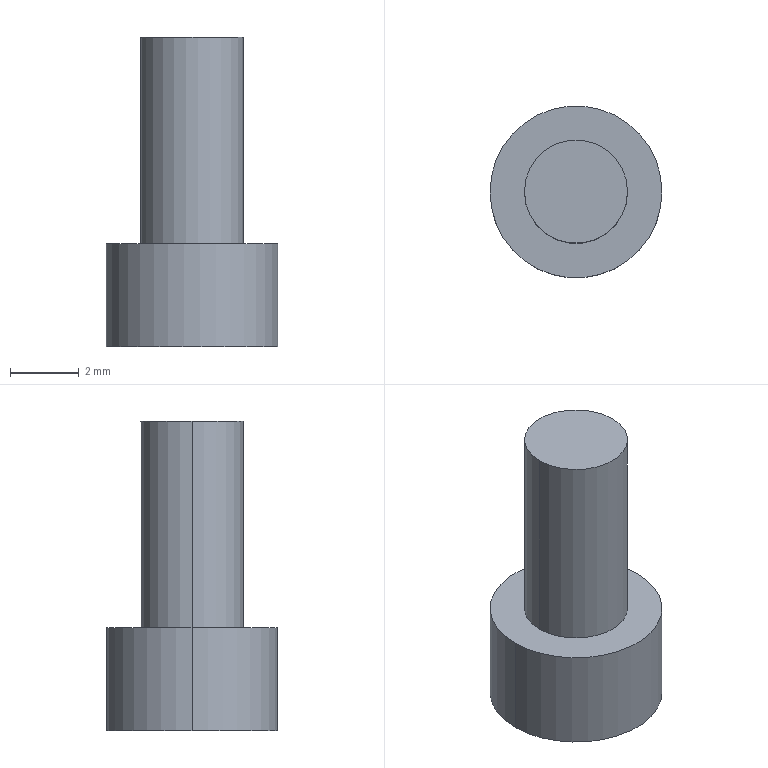Part | SolidWorks | features Extrusion 1, ICE 1 | 1 solid | 7 faces | box 5 x 5 x 9 mm | volume 101.316 mm3 | cylinder 4 | plane 3 | commonest cylinder face diameters 3 x2 5 x2
STEP:
#1=CARTESIAN_POINT('',(1.5,0.,9.));
#2=VERTEX_POINT('',#1);
#3=CARTESIAN_POINT('',(-1.5,0.,9.));
#4=VERTEX_POINT('',#3);
#5=CARTESIAN_POINT('',(0.,0.,9.));
#6=DIRECTION('',(0.,0.,1.));
#7=DIRECTION('',(1.,0.,0.));
#8=AXIS2_PLACEMENT_3D('',#5,#6,#7);
#9=CIRCLE('',#8,1.5);
#10=EDGE_CURVE('',#2,#4,#9,.T.);
#11=ORIENTED_EDGE('',*,*,#10,.F.);
#12=CARTESIAN_POINT('',(1.5,0.,3.));
#13=VERTEX_POINT('',#12);
#14=CARTESIAN_POINT('',(1.5,0.,9.));
#15=DIRECTION('',(0.,0.,-1.));
#16=VECTOR('',#15,1000.);
#17=LINE('',#14,#16);
#18=EDGE_CURVE('',#2,#13,#17,.T.);
#19=ORIENTED_EDGE('',*,*,#18,.T.);
#20=CARTESIAN_POINT('',(-1.5,0.,3.));
#21=VERTEX_POINT('',#20);
#22=CARTESIAN_POINT('',(0.,0.,3.));
#23=DIRECTION('',(0.,0.,1.));
#24=DIRECTION('',(1.,0.,0.));
#25=AXIS2_PLACEMENT_3D('',#22,#23,#24);
#26=CIRCLE('',#25,1.5);
#27=EDGE_CURVE('',#13,#21,#26,.T.);
#28=ORIENTED_EDGE('',*,*,#27,.T.);
#29=CARTESIAN_POINT('',(-1.5,0.,9.));
#30=DIRECTION('',(0.,0.,-1.));
#31=VECTOR('',#30,1000.);
#32=LINE('',#29,#31);
#33=EDGE_CURVE('',#4,#21,#32,.T.);
#34=ORIENTED_EDGE('',*,*,#33,.F.);
#35=EDGE_LOOP('',(#11,#19,#28,#34));
#36=FACE_OUTER_BOUND('',#35,.T.);
#37=CARTESIAN_POINT('',(0.,0.,9.));
#38=DIRECTION('',(0.,0.,-1.));
#39=DIRECTION('',(-1.,0.,0.));
#40=AXIS2_PLACEMENT_3D('',#37,#38,#39);
#41=CYLINDRICAL_SURFACE('',#40,1.5);
#42=ADVANCED_FACE('',(#36),#41,.T.);
#43=CARTESIAN_POINT('',(2.5,0.,3.));
#44=VERTEX_POINT('',#43);
#45=CARTESIAN_POINT('',(-2.5,0.,3.));
#46=VERTEX_POINT('',#45);
#47=CARTESIAN_POINT('',(0.,0.,3.));
#48=DIRECTION('',(0.,0.,1.));
#49=DIRECTION('',(1.,0.,0.));
#50=AXIS2_PLACEMENT_3D('',#47,#48,#49);
#51=CIRCLE('',#50,2.5);
#52=EDGE_CURVE('',#44,#46,#51,.T.);
#53=ORIENTED_EDGE('',*,*,#52,.F.);
#54=CARTESIAN_POINT('',(2.5,0.,0.));
#55=VERTEX_POINT('',#54);
#56=CARTESIAN_POINT('',(2.5,0.,3.));
#57=DIRECTION('',(0.,0.,-1.));
#58=VECTOR('',#57,1000.);
#59=LINE('',#56,#58);
#60=EDGE_CURVE('',#44,#55,#59,.T.);
#61=ORIENTED_EDGE('',*,*,#60,.T.);
#62=CARTESIAN_POINT('',(-2.5,0.,0.));
#63=VERTEX_POINT('',#62);
#64=CARTESIAN_POINT('',(0.,0.,0.));
#65=DIRECTION('',(0.,0.,1.));
#66=DIRECTION('',(1.,0.,0.));
#67=AXIS2_PLACEMENT_3D('',#64,#65,#66);
#68=CIRCLE('',#67,2.5);
#69=EDGE_CURVE('',#55,#63,#68,.T.);
#70=ORIENTED_EDGE('',*,*,#69,.T.);
#71=CARTESIAN_POINT('',(-2.5,0.,3.));
#72=DIRECTION('',(0.,0.,-1.));
#73=VECTOR('',#72,1000.);
#74=LINE('',#71,#73);
#75=EDGE_CURVE('',#46,#63,#74,.T.);
#76=ORIENTED_EDGE('',*,*,#75,.F.);
#77=EDGE_LOOP('',(#53,#61,#70,#76));
#78=FACE_OUTER_BOUND('',#77,.T.);
#79=CARTESIAN_POINT('',(0.,0.,3.));
#80=DIRECTION('',(0.,0.,-1.));
#81=DIRECTION('',(-1.,0.,0.));
#82=AXIS2_PLACEMENT_3D('',#79,#80,#81);
#83=CYLINDRICAL_SURFACE('',#82,2.5);
#84=ADVANCED_FACE('',(#78),#83,.T.);
#85=ORIENTED_EDGE('',*,*,#60,.F.);
#86=CARTESIAN_POINT('',(0.,0.,3.));
#87=DIRECTION('',(0.,0.,1.));
#88=DIRECTION('',(1.,0.,0.));
#89=AXIS2_PLACEMENT_3D('',#86,#87,#88);
#90=CIRCLE('',#89,2.5);
#91=EDGE_CURVE('',#46,#44,#90,.T.);
#92=ORIENTED_EDGE('',*,*,#91,.F.);
#93=ORIENTED_EDGE('',*,*,#75,.T.);
#94=CARTESIAN_POINT('',(0.,0.,0.));
#95=DIRECTION('',(0.,0.,1.));
#96=DIRECTION('',(1.,0.,0.));
#97=AXIS2_PLACEMENT_3D('',#94,#95,#96);
#98=CIRCLE('',#97,2.5);
#99=EDGE_CURVE('',#63,#55,#98,.T.);
#100=ORIENTED_EDGE('',*,*,#99,.T.);
#101=EDGE_LOOP('',(#85,#92,#93,#100));
#102=FACE_OUTER_BOUND('',#101,.T.);
#103=CARTESIAN_POINT('',(0.,0.,3.));
#104=DIRECTION('',(0.,0.,-1.));
#105=DIRECTION('',(-1.,0.,0.));
#106=AXIS2_PLACEMENT_3D('',#103,#104,#105);
#107=CYLINDRICAL_SURFACE('',#106,2.5);
#108=ADVANCED_FACE('',(#102),#107,.T.);
#109=CARTESIAN_POINT('',(0.,0.,3.));
#110=DIRECTION('',(0.,0.,1.));
#111=DIRECTION('',(1.,0.,0.));
#112=AXIS2_PLACEMENT_3D('',#109,#110,#111);
#113=CIRCLE('',#112,1.5);
#114=EDGE_CURVE('',#21,#13,#113,.T.);
#115=ORIENTED_EDGE('',*,*,#114,.F.);
#116=ORIENTED_EDGE('',*,*,#27,.F.);
#117=EDGE_LOOP('',(#115,#116));
#118=FACE_BOUND('',#117,.T.);
#119=ORIENTED_EDGE('',*,*,#91,.T.);
#120=ORIENTED_EDGE('',*,*,#52,.T.);
#121=EDGE_LOOP('',(#119,#120));
#122=FACE_OUTER_BOUND('',#121,.T.);
#123=CARTESIAN_POINT('',(0.,0.,3.));
#124=DIRECTION('',(0.,0.,1.));
#125=DIRECTION('',(1.,0.,0.));
#126=AXIS2_PLACEMENT_3D('',#123,#124,#125);
#127=PLANE('',#126);
#128=ADVANCED_FACE('',(#118,#122),#127,.T.);
#129=ORIENTED_EDGE('',*,*,#99,.F.);
#130=ORIENTED_EDGE('',*,*,#69,.F.);
#131=EDGE_LOOP('',(#129,#130));
#132=FACE_OUTER_BOUND('',#131,.T.);
#133=CARTESIAN_POINT('',(0.,0.,0.));
#134=DIRECTION('',(0.,0.,1.));
#135=DIRECTION('',(1.,0.,0.));
#136=AXIS2_PLACEMENT_3D('',#133,#134,#135);
#137=PLANE('',#136);
#138=ADVANCED_FACE('',(#132),#137,.F.);
#139=ORIENTED_EDGE('',*,*,#18,.F.);
#140=CARTESIAN_POINT('',(0.,0.,9.));
#141=DIRECTION('',(0.,0.,1.));
#142=DIRECTION('',(1.,0.,0.));
#143=AXIS2_PLACEMENT_3D('',#140,#141,#142);
#144=CIRCLE('',#143,1.5);
#145=EDGE_CURVE('',#4,#2,#144,.T.);
#146=ORIENTED_EDGE('',*,*,#145,.F.);
#147=ORIENTED_EDGE('',*,*,#33,.T.);
#148=ORIENTED_EDGE('',*,*,#114,.T.);
#149=EDGE_LOOP('',(#139,#146,#147,#148));
#150=FACE_OUTER_BOUND('',#149,.T.);
#151=CARTESIAN_POINT('',(0.,0.,9.));
#152=DIRECTION('',(0.,0.,-1.));
#153=DIRECTION('',(-1.,0.,0.));
#154=AXIS2_PLACEMENT_3D('',#151,#152,#153);
#155=CYLINDRICAL_SURFACE('',#154,1.5);
#156=ADVANCED_FACE('',(#150),#155,.T.);
#157=ORIENTED_EDGE('',*,*,#145,.T.);
#158=ORIENTED_EDGE('',*,*,#10,.T.);
#159=EDGE_LOOP('',(#157,#158));
#160=FACE_OUTER_BOUND('',#159,.T.);
#161=CARTESIAN_POINT('',(0.,0.,9.));
#162=DIRECTION('',(0.,0.,1.));
#163=DIRECTION('',(1.,0.,0.));
#164=AXIS2_PLACEMENT_3D('',#161,#162,#163);
#165=PLANE('',#164);
#166=ADVANCED_FACE('',(#160),#165,.T.);
#167=CLOSED_SHELL('',(#42,#84,#108,#128,#138,#156,#166));
#168=MANIFOLD_SOLID_BREP('',#167);
#169=CARTESIAN_POINT('',(0.,0.,0.));
#170=DIRECTION('',(0.,0.,1.));
#171=DIRECTION('',(1.,0.,0.));
#172=AXIS2_PLACEMENT_3D('',#169,#170,#171);
#173=(LENGTH_UNIT()NAMED_UNIT(*)SI_UNIT(.MILLI.,.METRE.));
#174=UNCERTAINTY_MEASURE_WITH_UNIT(LENGTH_MEASURE(0.00001),#173,'','');
#175=(NAMED_UNIT(*)PLANE_ANGLE_UNIT()SI_UNIT($,.RADIAN.));
#176=(NAMED_UNIT(*)SI_UNIT($,.STERADIAN.)SOLID_ANGLE_UNIT());
#177=(GEOMETRIC_REPRESENTATION_CONTEXT(3)GLOBAL_UNCERTAINTY_ASSIGNED_CONTEXT((#174))GLOBAL_UNIT_ASSIGNED_CONTEXT((#173,#175,#176))REPRESENTATION_CONTEXT('',''));
#178=ADVANCED_BREP_SHAPE_REPRESENTATION('',(#168,#172),#177);